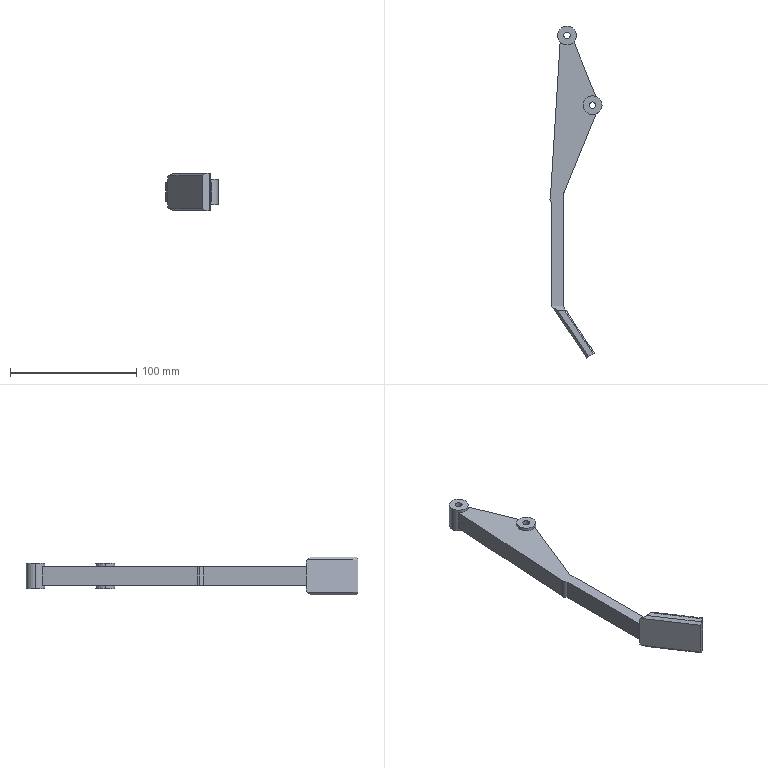Part | SolidWorks | features ICE 9, Chamfer 2, Extrusion 1 | 1 solid | 124 faces | box 41.169 x 262.682 x 30 mm | volume 65596 mm3 | plane 114 | cylinder 10 | commonest cylinder face diameters 5.2 x4 15 x4 8.722 x2